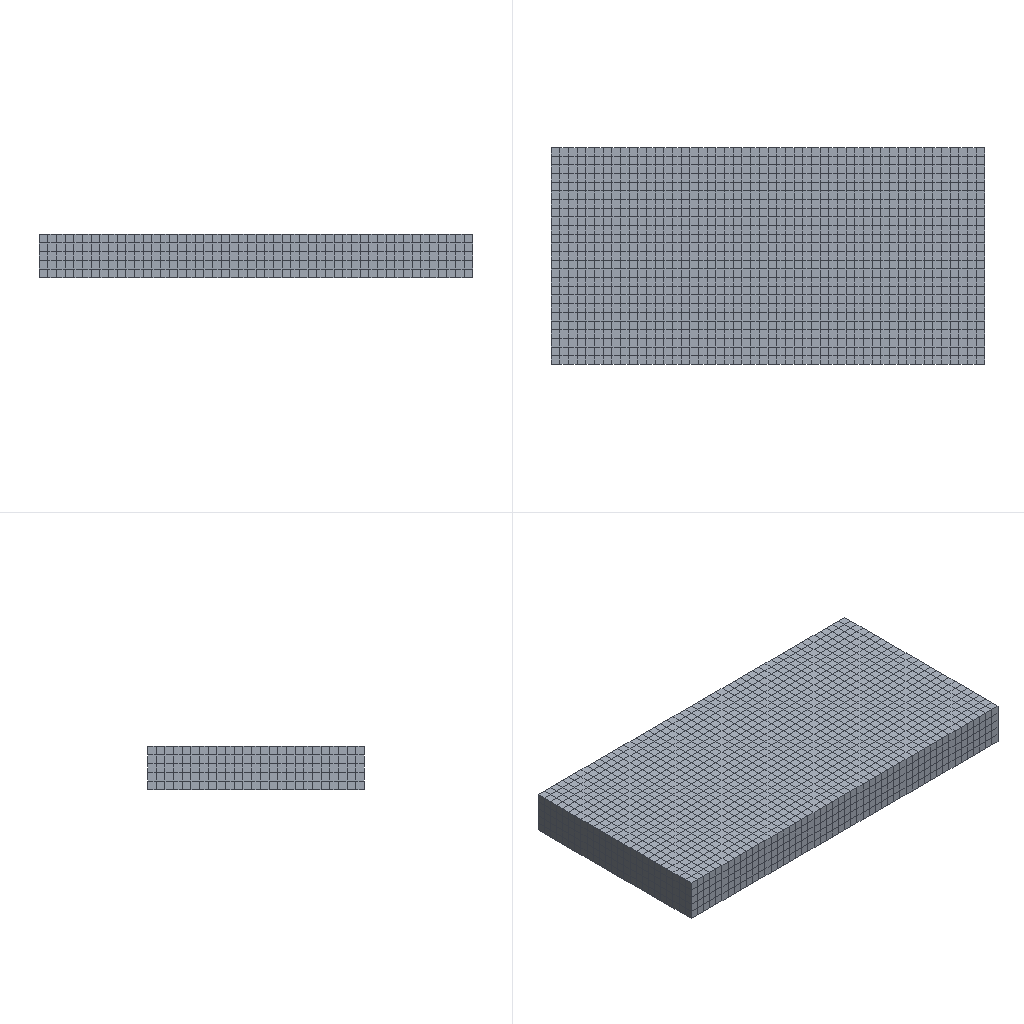Simulation study | abaqus
Set-up summary:
category,name,step,type,value,unit,region
solver,abaqus,,Abaqus/CAE 2024
units,mm-N-s-tonne (MPa),,inferred,E=72000 density=2.8e-09
analysis,Step-1,,dynamic explicit,nlgeom=True; time_period=0.01
analysis,Step-2,,dynamic explicit,nlgeom=True; time_period=0.01
analysis,Step-3,,dynamic explicit,nlgeom=True; time_period=0.01
analysis,Step-1,,dynamic explicit,nlgeom=True; time_period=0.01
analysis,Step-2,,dynamic explicit,nlgeom=True; time_period=0.01
analysis,Step-3,,dynamic explicit,nlgeom=True; time_period=0.01
analysis,Step-1,,dynamic explicit,nlgeom=True; time_period=0.01
analysis,Step-2,,dynamic explicit,nlgeom=True; time_period=0.01
analysis,Step-3,,dynamic explicit,nlgeom=True; time_period=0.01
mesh,deck-1.inp,,nodes,9381
mesh,deck-1.inp,,elements,7666
element_type,C3D8R,,,6250,,deck-1.inp
element_type,R3D4,,,1416,,deck-1.inp
mesh,deck-2.inp,,nodes,9381
mesh,deck-2.inp,,elements,7666
element_type,C3D8R,,,6250,,deck-2.inp
element_type,R3D4,,,1416,,deck-2.inp
mesh,deck-3.inp,,nodes,9381
mesh,deck-3.inp,,elements,7666
element_type,C3D8R,,,6250,,deck-3.inp
element_type,R3D4,,,1416,,deck-3.inp
material,Material-1,,E,72000
material,Material-1,,nu,0.3
material,Material-1,,density,2.8e-09
material,Material-1,,yield,200
material,Material-1,,behaviors,plastic; damage initiation; damage evolution
section,Material-1,,solid section,,,Set-1
section,Material-1,,solid section,,,Set-1
section,Material-1,,solid section,,,Set-1
bc,BC-fix,Step-1,encastre,[dofs=ENCASTRE n=3],,Set-1
bc,BC-v1,Step-1,velocity,"-5600 [dofs=rx,ry,rz,x,y,z n=18]",,Set-3
bc,BC-v2,Step-1,velocity,"[dofs=rx,ry,rz,x,y,z n=18]",,Set-4
bc,BC-v3,Step-1,velocity,"[dofs=rx,ry,rz,x,y,z n=18]",,Set-5
bc,BC-v1,Step-2,velocity,[dofs=x n=3],,Set-3
bc,BC-v2,Step-2,velocity,-5600 [dofs=x n=3],,Set-4
bc,BC-v2,Step-3,velocity,[dofs=x n=3],,Set-4
bc,BC-v3,Step-3,velocity,-5600 [dofs=x n=3],,Set-5
contact,Int-1,Step-1,contact pair,interaction=IntProp-1; friction=0.2; behavior=hard,,m_Surf-1 / s_Set-2_CNS_
contact,Int-1-Copy,Step-1,contact pair,interaction=IntProp-1; friction=0.2; behavior=hard,,m_Surf-2 / s_Set-2_CNS_
contact,Int-1-Copy2,Step-1,contact pair,interaction=IntProp-1; friction=0.2; behavior=hard,,m_Surf-3 / s_Set-2_CNS_
contact,Int-1,Step-1,contact pair,interaction=IntProp-1; friction=0.2; behavior=hard,,m_Surf-1 / s_Set-2_CNS_
contact,Int-1-Copy,Step-1,contact pair,interaction=IntProp-1; friction=0.2; behavior=hard,,m_Surf-2 / s_Set-2_CNS_
contact,Int-1-Copy2,Step-1,contact pair,interaction=IntProp-1; friction=0.2; behavior=hard,,m_Surf-3 / s_Set-2_CNS_
contact,Int-1,Step-1,contact pair,interaction=IntProp-1; friction=0.2; behavior=hard,,m_Surf-1 / s_Set-2_CNS_
contact,Int-1-Copy,Step-1,contact pair,interaction=IntProp-1; friction=0.2; behavior=hard,,m_Surf-2 / s_Set-2_CNS_
contact,Int-1-Copy2,Step-1,contact pair,interaction=IntProp-1; friction=0.2; behavior=hard,,m_Surf-3 / s_Set-2_CNS_
constraint,rigid body,,,9
Results summary:
result,odb.job_status,,,JOB_STATUS_COMPLETED_SUCCESSFULLY,"consistent, unstated (Abaqus has no unit system)"
result,steps[0].procedure,Step-1,,"*DYNAMIC, EXPLICIT","consistent, unstated (Abaqus has no unit system)"
result,steps[0].time_period,Step-1,,0.01,"consistent, unstated (Abaqus has no unit system)"
result,steps[0].n_frames,Step-1,,41,"consistent, unstated (Abaqus has no unit system)"
result,steps[0].last_frame.id,Step-1,,3157,"consistent, unstated (Abaqus has no unit system)"
result,steps[0].last_frame.value,Step-1,,0.01,"consistent, unstated (Abaqus has no unit system)"
result,steps[0].last_frame.description,Step-1,,Increment      3157: Step Time =   1.0000E-02,"consistent, unstated (Abaqus has no unit system)"
result,steps[0].completed,Step-1,,True,"consistent, unstated (Abaqus has no unit system)"
result,steps[0].max_U_magnitude,Step-1,,62.517,"consistent, unstated (Abaqus has no unit system)"
result,steps[0].max_S_mises,Step-1,,112.257,"consistent, unstated (Abaqus has no unit system)"
result,steps[0].RF_sum[1],Step-1,,1620.44,"consistent, unstated (Abaqus has no unit system)"
result,steps[0].RF_sum[2],Step-1,,-10.971,"consistent, unstated (Abaqus has no unit system)"
result,steps[0].RF_sum[3],Step-1,,655.379,"consistent, unstated (Abaqus has no unit system)"
result,steps[0].diagnostic.n_increments,Step-1,,41,"consistent, unstated (Abaqus has no unit system)"
result,steps[1].procedure,Step-2,,"*DYNAMIC, EXPLICIT","consistent, unstated (Abaqus has no unit system)"
result,steps[1].time_period,Step-2,,0.01,"consistent, unstated (Abaqus has no unit system)"
result,steps[1].n_frames,Step-2,,41,"consistent, unstated (Abaqus has no unit system)"
result,steps[1].last_frame.id,Step-2,,3156,"consistent, unstated (Abaqus has no unit system)"
result,steps[1].last_frame.value,Step-2,,0.01,"consistent, unstated (Abaqus has no unit system)"
result,steps[1].last_frame.description,Step-2,,Increment      3156: Step Time =   1.0000E-02,"consistent, unstated (Abaqus has no unit system)"
result,steps[1].completed,Step-2,,True,"consistent, unstated (Abaqus has no unit system)"
result,steps[1].max_U_magnitude,Step-2,,125.845,"consistent, unstated (Abaqus has no unit system)"
result,steps[1].max_S_mises,Step-2,,146.03,"consistent, unstated (Abaqus has no unit system)"
result,steps[1].RF_sum[1],Step-2,,1586.31,"consistent, unstated (Abaqus has no unit system)"
result,steps[1].RF_sum[2],Step-2,,2574.8,"consistent, unstated (Abaqus has no unit system)"
result,steps[1].RF_sum[3],Step-2,,223.696,"consistent, unstated (Abaqus has no unit system)"
result,steps[1].diagnostic.n_increments,Step-2,,41,"consistent, unstated (Abaqus has no unit system)"
result,steps[2].procedure,Step-3,,"*DYNAMIC, EXPLICIT","consistent, unstated (Abaqus has no unit system)"
result,steps[2].time_period,Step-3,,0.01,"consistent, unstated (Abaqus has no unit system)"
result,steps[2].n_frames,Step-3,,41,"consistent, unstated (Abaqus has no unit system)"
result,steps[2].last_frame.id,Step-3,,3160,"consistent, unstated (Abaqus has no unit system)"
result,steps[2].last_frame.value,Step-3,,0.01,"consistent, unstated (Abaqus has no unit system)"
result,steps[2].last_frame.description,Step-3,,Increment      3160: Step Time =   1.0000E-02,"consistent, unstated (Abaqus has no unit system)"
result,steps[2].completed,Step-3,,True,"consistent, unstated (Abaqus has no unit system)"
result,steps[2].max_U_magnitude,Step-3,,189.343,"consistent, unstated (Abaqus has no unit system)"
result,steps[2].max_S_mises,Step-3,,127.55,"consistent, unstated (Abaqus has no unit system)"
result,steps[2].RF_sum[1],Step-3,,-1799.44,"consistent, unstated (Abaqus has no unit system)"
result,steps[2].RF_sum[2],Step-3,,151.63,"consistent, unstated (Abaqus has no unit system)"
result,steps[2].RF_sum[3],Step-3,,-16.143,"consistent, unstated (Abaqus has no unit system)"
result,steps[2].diagnostic.n_increments,Step-3,,41,"consistent, unstated (Abaqus has no unit system)"